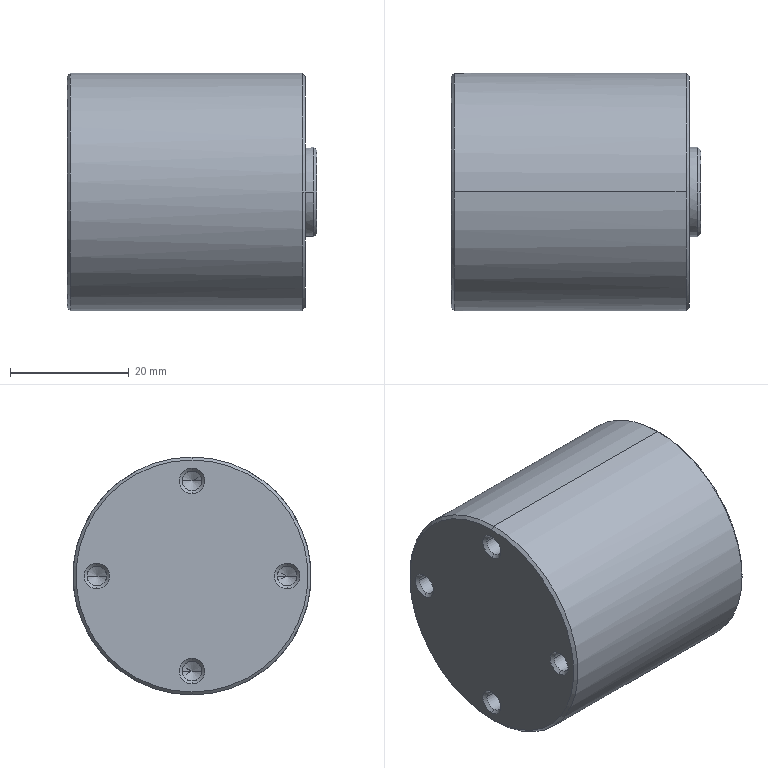Part | STEP file | 05-05 Fixture | 1 solid | 42 faces | box 42 x 40 x 40 mm | volume 49529 mm3 | cone 24 | cylinder 14 | plane 4 | commonest cylinder face diameters 3.3 x8 10 x2 15 x2 40 x2